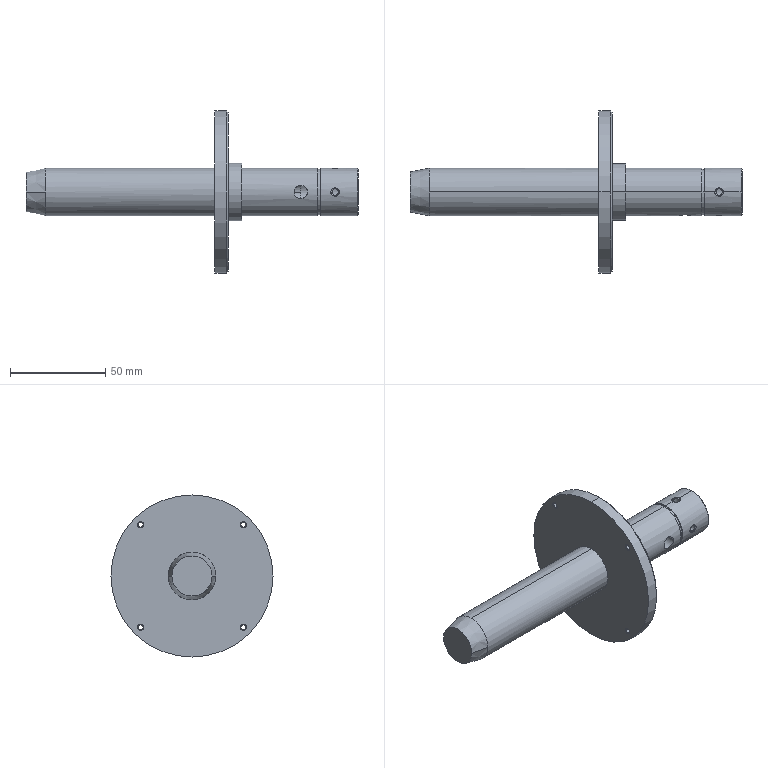Part | NX | 1 solid | 60 faces | box 174 x 85 x 85 mm | volume 118428 mm3 | cylinder 29 | cone 16 | plane 11 | spline 4 | commonest cylinder face diameters 2.5 x8 25 x6 3.3 x4 7 x2 9 x2 23.9 x2